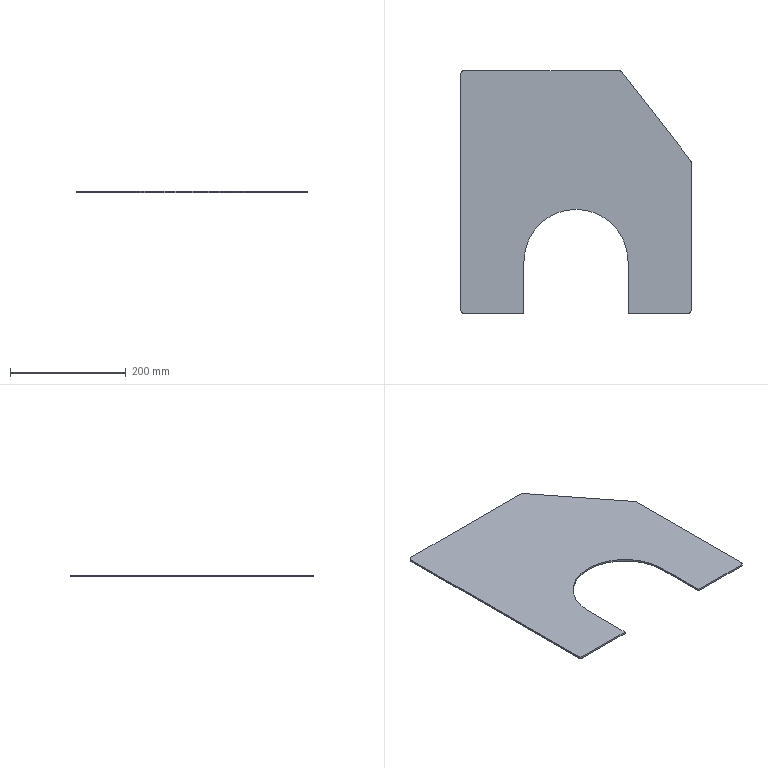Part | SolidWorks | features Extrusion 1 | 1 solid | 16 faces | box 398 x 420 x 3 mm | volume 386101 mm3 | plane 10 | cylinder 6 | commonest cylinder face diameters 10 x5 180 x1
STEP:
#1=CARTESIAN_POINT('',(0.,5.,0.));
#2=VERTEX_POINT('',#1);
#3=CARTESIAN_POINT('',(5.,0.,0.));
#4=VERTEX_POINT('',#3);
#5=CARTESIAN_POINT('',(5.,5.,0.));
#6=DIRECTION('',(0.,0.,1.));
#7=DIRECTION('',(1.,0.,0.));
#8=AXIS2_PLACEMENT_3D('',#5,#6,#7);
#9=CIRCLE('',#8,5.);
#10=EDGE_CURVE('',#2,#4,#9,.T.);
#11=ORIENTED_EDGE('',*,*,#10,.T.);
#12=CARTESIAN_POINT('',(5.,0.,3.));
#13=VERTEX_POINT('',#12);
#14=CARTESIAN_POINT('',(5.,0.,3.));
#15=DIRECTION('',(0.,0.,-1.));
#16=VECTOR('',#15,1000.);
#17=LINE('',#14,#16);
#18=EDGE_CURVE('',#13,#4,#17,.T.);
#19=ORIENTED_EDGE('',*,*,#18,.F.);
#20=CARTESIAN_POINT('',(0.,5.,3.));
#21=VERTEX_POINT('',#20);
#22=CARTESIAN_POINT('',(5.,5.,3.));
#23=DIRECTION('',(0.,0.,1.));
#24=DIRECTION('',(1.,0.,0.));
#25=AXIS2_PLACEMENT_3D('',#22,#23,#24);
#26=CIRCLE('',#25,5.);
#27=EDGE_CURVE('',#21,#13,#26,.T.);
#28=ORIENTED_EDGE('',*,*,#27,.F.);
#29=CARTESIAN_POINT('',(0.,5.,3.));
#30=DIRECTION('',(0.,0.,-1.));
#31=VECTOR('',#30,1000.);
#32=LINE('',#29,#31);
#33=EDGE_CURVE('',#21,#2,#32,.T.);
#34=ORIENTED_EDGE('',*,*,#33,.T.);
#35=EDGE_LOOP('',(#11,#19,#28,#34));
#36=FACE_OUTER_BOUND('',#35,.T.);
#37=CARTESIAN_POINT('',(5.,5.,3.));
#38=DIRECTION('',(0.,0.,-1.));
#39=DIRECTION('',(-1.,0.,0.));
#40=AXIS2_PLACEMENT_3D('',#37,#38,#39);
#41=CYLINDRICAL_SURFACE('',#40,5.);
#42=ADVANCED_FACE('',(#36),#41,.T.);
#43=CARTESIAN_POINT('',(109.,0.,0.));
#44=VERTEX_POINT('',#43);
#45=CARTESIAN_POINT('',(109.,0.,0.));
#46=DIRECTION('',(1.,0.,0.));
#47=VECTOR('',#46,1000.);
#48=LINE('',#45,#47);
#49=EDGE_CURVE('',#4,#44,#48,.T.);
#50=ORIENTED_EDGE('',*,*,#49,.T.);
#51=CARTESIAN_POINT('',(109.,0.,3.));
#52=VERTEX_POINT('',#51);
#53=CARTESIAN_POINT('',(109.,0.,3.));
#54=DIRECTION('',(0.,0.,-1.));
#55=VECTOR('',#54,1000.);
#56=LINE('',#53,#55);
#57=EDGE_CURVE('',#52,#44,#56,.T.);
#58=ORIENTED_EDGE('',*,*,#57,.F.);
#59=CARTESIAN_POINT('',(109.,0.,3.));
#60=DIRECTION('',(1.,0.,0.));
#61=VECTOR('',#60,1000.);
#62=LINE('',#59,#61);
#63=EDGE_CURVE('',#13,#52,#62,.T.);
#64=ORIENTED_EDGE('',*,*,#63,.F.);
#65=ORIENTED_EDGE('',*,*,#18,.T.);
#66=EDGE_LOOP('',(#50,#58,#64,#65));
#67=FACE_OUTER_BOUND('',#66,.T.);
#68=CARTESIAN_POINT('',(109.,0.,3.));
#69=DIRECTION('',(0.,1.,0.));
#70=DIRECTION('',(-1.,0.,0.));
#71=AXIS2_PLACEMENT_3D('',#68,#69,#70);
#72=PLANE('',#71);
#73=ADVANCED_FACE('',(#67),#72,.F.);
#74=CARTESIAN_POINT('',(109.,90.,0.));
#75=VERTEX_POINT('',#74);
#76=CARTESIAN_POINT('',(109.,90.,0.));
#77=DIRECTION('',(0.,1.,0.));
#78=VECTOR('',#77,1000.);
#79=LINE('',#76,#78);
#80=EDGE_CURVE('',#44,#75,#79,.T.);
#81=ORIENTED_EDGE('',*,*,#80,.T.);
#82=CARTESIAN_POINT('',(109.,90.,3.));
#83=VERTEX_POINT('',#82);
#84=CARTESIAN_POINT('',(109.,90.,3.));
#85=DIRECTION('',(0.,0.,-1.));
#86=VECTOR('',#85,1000.);
#87=LINE('',#84,#86);
#88=EDGE_CURVE('',#83,#75,#87,.T.);
#89=ORIENTED_EDGE('',*,*,#88,.F.);
#90=CARTESIAN_POINT('',(109.,90.,3.));
#91=DIRECTION('',(0.,1.,0.));
#92=VECTOR('',#91,1000.);
#93=LINE('',#90,#92);
#94=EDGE_CURVE('',#52,#83,#93,.T.);
#95=ORIENTED_EDGE('',*,*,#94,.F.);
#96=ORIENTED_EDGE('',*,*,#57,.T.);
#97=EDGE_LOOP('',(#81,#89,#95,#96));
#98=FACE_OUTER_BOUND('',#97,.T.);
#99=CARTESIAN_POINT('',(109.,90.,3.));
#100=DIRECTION('',(-1.,0.,0.));
#101=DIRECTION('',(0.,-1.,0.));
#102=AXIS2_PLACEMENT_3D('',#99,#100,#101);
#103=PLANE('',#102);
#104=ADVANCED_FACE('',(#98),#103,.F.);
#105=CARTESIAN_POINT('',(289.,90.,0.));
#106=VERTEX_POINT('',#105);
#107=CARTESIAN_POINT('',(199.,90.,0.));
#108=DIRECTION('',(0.,0.,-1.));
#109=DIRECTION('',(1.,0.,0.));
#110=AXIS2_PLACEMENT_3D('',#107,#108,#109);
#111=CIRCLE('',#110,90.);
#112=EDGE_CURVE('',#75,#106,#111,.T.);
#113=ORIENTED_EDGE('',*,*,#112,.T.);
#114=CARTESIAN_POINT('',(289.,90.,3.));
#115=VERTEX_POINT('',#114);
#116=CARTESIAN_POINT('',(289.,90.,3.));
#117=DIRECTION('',(0.,0.,-1.));
#118=VECTOR('',#117,1000.);
#119=LINE('',#116,#118);
#120=EDGE_CURVE('',#115,#106,#119,.T.);
#121=ORIENTED_EDGE('',*,*,#120,.F.);
#122=CARTESIAN_POINT('',(199.,90.,3.));
#123=DIRECTION('',(0.,0.,-1.));
#124=DIRECTION('',(1.,0.,0.));
#125=AXIS2_PLACEMENT_3D('',#122,#123,#124);
#126=CIRCLE('',#125,90.);
#127=EDGE_CURVE('',#83,#115,#126,.T.);
#128=ORIENTED_EDGE('',*,*,#127,.F.);
#129=ORIENTED_EDGE('',*,*,#88,.T.);
#130=EDGE_LOOP('',(#113,#121,#128,#129));
#131=FACE_OUTER_BOUND('',#130,.T.);
#132=CARTESIAN_POINT('',(199.,90.,3.));
#133=DIRECTION('',(0.,0.,-1.));
#134=DIRECTION('',(-1.,0.,0.));
#135=AXIS2_PLACEMENT_3D('',#132,#133,#134);
#136=CYLINDRICAL_SURFACE('',#135,90.);
#137=ADVANCED_FACE('',(#131),#136,.F.);
#138=CARTESIAN_POINT('',(289.,0.,0.));
#139=VERTEX_POINT('',#138);
#140=CARTESIAN_POINT('',(289.,90.,0.));
#141=DIRECTION('',(0.,-1.,0.));
#142=VECTOR('',#141,1000.);
#143=LINE('',#140,#142);
#144=EDGE_CURVE('',#106,#139,#143,.T.);
#145=ORIENTED_EDGE('',*,*,#144,.T.);
#146=CARTESIAN_POINT('',(289.,0.,3.));
#147=VERTEX_POINT('',#146);
#148=CARTESIAN_POINT('',(289.,0.,3.));
#149=DIRECTION('',(0.,0.,-1.));
#150=VECTOR('',#149,1000.);
#151=LINE('',#148,#150);
#152=EDGE_CURVE('',#147,#139,#151,.T.);
#153=ORIENTED_EDGE('',*,*,#152,.F.);
#154=CARTESIAN_POINT('',(289.,90.,3.));
#155=DIRECTION('',(0.,-1.,0.));
#156=VECTOR('',#155,1000.);
#157=LINE('',#154,#156);
#158=EDGE_CURVE('',#115,#147,#157,.T.);
#159=ORIENTED_EDGE('',*,*,#158,.F.);
#160=ORIENTED_EDGE('',*,*,#120,.T.);
#161=EDGE_LOOP('',(#145,#153,#159,#160));
#162=FACE_OUTER_BOUND('',#161,.T.);
#163=CARTESIAN_POINT('',(289.,90.,3.));
#164=DIRECTION('',(1.,0.,0.));
#165=DIRECTION('',(0.,0.,-1.));
#166=AXIS2_PLACEMENT_3D('',#163,#164,#165);
#167=PLANE('',#166);
#168=ADVANCED_FACE('',(#162),#167,.F.);
#169=CARTESIAN_POINT('',(393.,0.,0.));
#170=VERTEX_POINT('',#169);
#171=CARTESIAN_POINT('',(393.,0.,0.));
#172=DIRECTION('',(1.,0.,0.));
#173=VECTOR('',#172,1000.);
#174=LINE('',#171,#173);
#175=EDGE_CURVE('',#139,#170,#174,.T.);
#176=ORIENTED_EDGE('',*,*,#175,.T.);
#177=CARTESIAN_POINT('',(393.,0.,3.));
#178=VERTEX_POINT('',#177);
#179=CARTESIAN_POINT('',(393.,0.,3.));
#180=DIRECTION('',(0.,0.,-1.));
#181=VECTOR('',#180,1000.);
#182=LINE('',#179,#181);
#183=EDGE_CURVE('',#178,#170,#182,.T.);
#184=ORIENTED_EDGE('',*,*,#183,.F.);
#185=CARTESIAN_POINT('',(393.,0.,3.));
#186=DIRECTION('',(1.,0.,0.));
#187=VECTOR('',#186,1000.);
#188=LINE('',#185,#187);
#189=EDGE_CURVE('',#147,#178,#188,.T.);
#190=ORIENTED_EDGE('',*,*,#189,.F.);
#191=ORIENTED_EDGE('',*,*,#152,.T.);
#192=EDGE_LOOP('',(#176,#184,#190,#191));
#193=FACE_OUTER_BOUND('',#192,.T.);
#194=CARTESIAN_POINT('',(393.,0.,3.));
#195=DIRECTION('',(0.,1.,0.));
#196=DIRECTION('',(-1.,0.,0.));
#197=AXIS2_PLACEMENT_3D('',#194,#195,#196);
#198=PLANE('',#197);
#199=ADVANCED_FACE('',(#193),#198,.F.);
#200=CARTESIAN_POINT('',(398.,5.,0.));
#201=VERTEX_POINT('',#200);
#202=CARTESIAN_POINT('',(393.,5.,0.));
#203=DIRECTION('',(0.,0.,1.));
#204=DIRECTION('',(-1.,0.,0.));
#205=AXIS2_PLACEMENT_3D('',#202,#203,#204);
#206=CIRCLE('',#205,5.);
#207=EDGE_CURVE('',#170,#201,#206,.T.);
#208=ORIENTED_EDGE('',*,*,#207,.T.);
#209=CARTESIAN_POINT('',(398.,5.,3.));
#210=VERTEX_POINT('',#209);
#211=CARTESIAN_POINT('',(398.,5.,3.));
#212=DIRECTION('',(0.,0.,-1.));
#213=VECTOR('',#212,1000.);
#214=LINE('',#211,#213);
#215=EDGE_CURVE('',#210,#201,#214,.T.);
#216=ORIENTED_EDGE('',*,*,#215,.F.);
#217=CARTESIAN_POINT('',(393.,5.,3.));
#218=DIRECTION('',(0.,0.,1.));
#219=DIRECTION('',(-1.,0.,0.));
#220=AXIS2_PLACEMENT_3D('',#217,#218,#219);
#221=CIRCLE('',#220,5.);
#222=EDGE_CURVE('',#178,#210,#221,.T.);
#223=ORIENTED_EDGE('',*,*,#222,.F.);
#224=ORIENTED_EDGE('',*,*,#183,.T.);
#225=EDGE_LOOP('',(#208,#216,#223,#224));
#226=FACE_OUTER_BOUND('',#225,.T.);
#227=CARTESIAN_POINT('',(393.,5.,3.));
#228=DIRECTION('',(0.,0.,-1.));
#229=DIRECTION('',(-1.,0.,0.));
#230=AXIS2_PLACEMENT_3D('',#227,#228,#229);
#231=CYLINDRICAL_SURFACE('',#230,5.);
#232=ADVANCED_FACE('',(#226),#231,.T.);
#233=CARTESIAN_POINT('',(398.,262.178,0.));
#234=VERTEX_POINT('',#233);
#235=CARTESIAN_POINT('',(398.,262.178,0.));
#236=DIRECTION('',(0.,1.,0.));
#237=VECTOR('',#236,1000.);
#238=LINE('',#235,#237);
#239=EDGE_CURVE('',#201,#234,#238,.T.);
#240=ORIENTED_EDGE('',*,*,#239,.T.);
#241=CARTESIAN_POINT('',(398.,262.178,3.));
#242=VERTEX_POINT('',#241);
#243=CARTESIAN_POINT('',(398.,262.178,3.));
#244=DIRECTION('',(0.,0.,-1.));
#245=VECTOR('',#244,1000.);
#246=LINE('',#243,#245);
#247=EDGE_CURVE('',#242,#234,#246,.T.);
#248=ORIENTED_EDGE('',*,*,#247,.F.);
#249=CARTESIAN_POINT('',(398.,262.178,3.));
#250=DIRECTION('',(0.,1.,0.));
#251=VECTOR('',#250,1000.);
#252=LINE('',#249,#251);
#253=EDGE_CURVE('',#210,#242,#252,.T.);
#254=ORIENTED_EDGE('',*,*,#253,.F.);
#255=ORIENTED_EDGE('',*,*,#215,.T.);
#256=EDGE_LOOP('',(#240,#248,#254,#255));
#257=FACE_OUTER_BOUND('',#256,.T.);
#258=CARTESIAN_POINT('',(398.,262.178,3.));
#259=DIRECTION('',(-1.,0.,0.));
#260=DIRECTION('',(0.,-1.,0.));
#261=AXIS2_PLACEMENT_3D('',#258,#259,#260);
#262=PLANE('',#261);
#263=ADVANCED_FACE('',(#257),#262,.F.);
#264=CARTESIAN_POINT('',(396.94,265.257,0.));
#265=VERTEX_POINT('',#264);
#266=CARTESIAN_POINT('',(393.,262.178,0.));
#267=DIRECTION('',(0.,0.,1.));
#268=DIRECTION('',(-1.,0.,0.));
#269=AXIS2_PLACEMENT_3D('',#266,#267,#268);
#270=CIRCLE('',#269,5.);
#271=EDGE_CURVE('',#234,#265,#270,.T.);
#272=ORIENTED_EDGE('',*,*,#271,.T.);
#273=CARTESIAN_POINT('',(396.94,265.257,3.));
#274=VERTEX_POINT('',#273);
#275=CARTESIAN_POINT('',(396.94,265.257,3.));
#276=DIRECTION('',(0.,0.,-1.));
#277=VECTOR('',#276,1000.);
#278=LINE('',#275,#277);
#279=EDGE_CURVE('',#274,#265,#278,.T.);
#280=ORIENTED_EDGE('',*,*,#279,.F.);
#281=CARTESIAN_POINT('',(393.,262.178,3.));
#282=DIRECTION('',(0.,0.,1.));
#283=DIRECTION('',(-1.,0.,0.));
#284=AXIS2_PLACEMENT_3D('',#281,#282,#283);
#285=CIRCLE('',#284,5.);
#286=EDGE_CURVE('',#242,#274,#285,.T.);
#287=ORIENTED_EDGE('',*,*,#286,.F.);
#288=ORIENTED_EDGE('',*,*,#247,.T.);
#289=EDGE_LOOP('',(#272,#280,#287,#288));
#290=FACE_OUTER_BOUND('',#289,.T.);
#291=CARTESIAN_POINT('',(393.,262.178,3.));
#292=DIRECTION('',(0.,0.,-1.));
#293=DIRECTION('',(-1.,0.,0.));
#294=AXIS2_PLACEMENT_3D('',#291,#292,#293);
#295=CYLINDRICAL_SURFACE('',#294,5.);
#296=ADVANCED_FACE('',(#290),#295,.T.);
#297=CARTESIAN_POINT('',(277.543,418.078,0.));
#298=VERTEX_POINT('',#297);
#299=CARTESIAN_POINT('',(277.543,418.078,0.));
#300=DIRECTION('',(-0.6157,0.788,0.));
#301=VECTOR('',#300,1000.);
#302=LINE('',#299,#301);
#303=EDGE_CURVE('',#265,#298,#302,.T.);
#304=ORIENTED_EDGE('',*,*,#303,.T.);
#305=CARTESIAN_POINT('',(277.543,418.078,3.));
#306=VERTEX_POINT('',#305);
#307=CARTESIAN_POINT('',(277.543,418.078,3.));
#308=DIRECTION('',(0.,0.,-1.));
#309=VECTOR('',#308,1000.);
#310=LINE('',#307,#309);
#311=EDGE_CURVE('',#306,#298,#310,.T.);
#312=ORIENTED_EDGE('',*,*,#311,.F.);
#313=CARTESIAN_POINT('',(277.543,418.078,3.));
#314=DIRECTION('',(-0.6157,0.788,0.));
#315=VECTOR('',#314,1000.);
#316=LINE('',#313,#315);
#317=EDGE_CURVE('',#274,#306,#316,.T.);
#318=ORIENTED_EDGE('',*,*,#317,.F.);
#319=ORIENTED_EDGE('',*,*,#279,.T.);
#320=EDGE_LOOP('',(#304,#312,#318,#319));
#321=FACE_OUTER_BOUND('',#320,.T.);
#322=CARTESIAN_POINT('',(277.543,418.078,3.));
#323=DIRECTION('',(-0.788,-0.6157,0.));
#324=DIRECTION('',(0.6157,-0.788,0.));
#325=AXIS2_PLACEMENT_3D('',#322,#323,#324);
#326=PLANE('',#325);
#327=ADVANCED_FACE('',(#321),#326,.F.);
#328=CARTESIAN_POINT('',(273.603,420.,0.));
#329=VERTEX_POINT('',#328);
#330=CARTESIAN_POINT('',(273.603,415.,0.));
#331=DIRECTION('',(0.,0.,1.));
#332=DIRECTION('',(-1.,0.,0.));
#333=AXIS2_PLACEMENT_3D('',#330,#331,#332);
#334=CIRCLE('',#333,5.);
#335=EDGE_CURVE('',#298,#329,#334,.T.);
#336=ORIENTED_EDGE('',*,*,#335,.T.);
#337=CARTESIAN_POINT('',(273.603,420.,3.));
#338=VERTEX_POINT('',#337);
#339=CARTESIAN_POINT('',(273.603,420.,3.));
#340=DIRECTION('',(0.,0.,-1.));
#341=VECTOR('',#340,1000.);
#342=LINE('',#339,#341);
#343=EDGE_CURVE('',#338,#329,#342,.T.);
#344=ORIENTED_EDGE('',*,*,#343,.F.);
#345=CARTESIAN_POINT('',(273.603,415.,3.));
#346=DIRECTION('',(0.,0.,1.));
#347=DIRECTION('',(-1.,0.,0.));
#348=AXIS2_PLACEMENT_3D('',#345,#346,#347);
#349=CIRCLE('',#348,5.);
#350=EDGE_CURVE('',#306,#338,#349,.T.);
#351=ORIENTED_EDGE('',*,*,#350,.F.);
#352=ORIENTED_EDGE('',*,*,#311,.T.);
#353=EDGE_LOOP('',(#336,#344,#351,#352));
#354=FACE_OUTER_BOUND('',#353,.T.);
#355=CARTESIAN_POINT('',(273.603,415.,3.));
#356=DIRECTION('',(0.,0.,-1.));
#357=DIRECTION('',(-1.,0.,0.));
#358=AXIS2_PLACEMENT_3D('',#355,#356,#357);
#359=CYLINDRICAL_SURFACE('',#358,5.);
#360=ADVANCED_FACE('',(#354),#359,.T.);
#361=CARTESIAN_POINT('',(5.,420.,0.));
#362=VERTEX_POINT('',#361);
#363=CARTESIAN_POINT('',(5.,420.,0.));
#364=DIRECTION('',(-1.,0.,0.));
#365=VECTOR('',#364,1000.);
#366=LINE('',#363,#365);
#367=EDGE_CURVE('',#329,#362,#366,.T.);
#368=ORIENTED_EDGE('',*,*,#367,.T.);
#369=CARTESIAN_POINT('',(5.,420.,3.));
#370=VERTEX_POINT('',#369);
#371=CARTESIAN_POINT('',(5.,420.,3.));
#372=DIRECTION('',(0.,0.,-1.));
#373=VECTOR('',#372,1000.);
#374=LINE('',#371,#373);
#375=EDGE_CURVE('',#370,#362,#374,.T.);
#376=ORIENTED_EDGE('',*,*,#375,.F.);
#377=CARTESIAN_POINT('',(5.,420.,3.));
#378=DIRECTION('',(-1.,0.,0.));
#379=VECTOR('',#378,1000.);
#380=LINE('',#377,#379);
#381=EDGE_CURVE('',#338,#370,#380,.T.);
#382=ORIENTED_EDGE('',*,*,#381,.F.);
#383=ORIENTED_EDGE('',*,*,#343,.T.);
#384=EDGE_LOOP('',(#368,#376,#382,#383));
#385=FACE_OUTER_BOUND('',#384,.T.);
#386=CARTESIAN_POINT('',(5.,420.,3.));
#387=DIRECTION('',(0.,-1.,0.));
#388=DIRECTION('',(0.,0.,-1.));
#389=AXIS2_PLACEMENT_3D('',#386,#387,#388);
#390=PLANE('',#389);
#391=ADVANCED_FACE('',(#385),#390,.F.);
#392=CARTESIAN_POINT('',(0.,415.,0.));
#393=VERTEX_POINT('',#392);
#394=CARTESIAN_POINT('',(5.,415.,0.));
#395=DIRECTION('',(0.,0.,1.));
#396=DIRECTION('',(-1.,0.,0.));
#397=AXIS2_PLACEMENT_3D('',#394,#395,#396);
#398=CIRCLE('',#397,5.);
#399=EDGE_CURVE('',#362,#393,#398,.T.);
#400=ORIENTED_EDGE('',*,*,#399,.T.);
#401=CARTESIAN_POINT('',(0.,415.,3.));
#402=VERTEX_POINT('',#401);
#403=CARTESIAN_POINT('',(0.,415.,3.));
#404=DIRECTION('',(0.,0.,-1.));
#405=VECTOR('',#404,1000.);
#406=LINE('',#403,#405);
#407=EDGE_CURVE('',#402,#393,#406,.T.);
#408=ORIENTED_EDGE('',*,*,#407,.F.);
#409=CARTESIAN_POINT('',(5.,415.,3.));
#410=DIRECTION('',(0.,0.,1.));
#411=DIRECTION('',(-1.,0.,0.));
#412=AXIS2_PLACEMENT_3D('',#409,#410,#411);
#413=CIRCLE('',#412,5.);
#414=EDGE_CURVE('',#370,#402,#413,.T.);
#415=ORIENTED_EDGE('',*,*,#414,.F.);
#416=ORIENTED_EDGE('',*,*,#375,.T.);
#417=EDGE_LOOP('',(#400,#408,#415,#416));
#418=FACE_OUTER_BOUND('',#417,.T.);
#419=CARTESIAN_POINT('',(5.,415.,3.));
#420=DIRECTION('',(0.,0.,-1.));
#421=DIRECTION('',(-1.,0.,0.));
#422=AXIS2_PLACEMENT_3D('',#419,#420,#421);
#423=CYLINDRICAL_SURFACE('',#422,5.);
#424=ADVANCED_FACE('',(#418),#423,.T.);
#425=CARTESIAN_POINT('',(0.,5.,0.));
#426=DIRECTION('',(0.,-1.,0.));
#427=VECTOR('',#426,1000.);
#428=LINE('',#425,#427);
#429=EDGE_CURVE('',#393,#2,#428,.T.);
#430=ORIENTED_EDGE('',*,*,#429,.T.);
#431=ORIENTED_EDGE('',*,*,#33,.F.);
#432=CARTESIAN_POINT('',(0.,5.,3.));
#433=DIRECTION('',(0.,-1.,0.));
#434=VECTOR('',#433,1000.);
#435=LINE('',#432,#434);
#436=EDGE_CURVE('',#402,#21,#435,.T.);
#437=ORIENTED_EDGE('',*,*,#436,.F.);
#438=ORIENTED_EDGE('',*,*,#407,.T.);
#439=EDGE_LOOP('',(#430,#431,#437,#438));
#440=FACE_OUTER_BOUND('',#439,.T.);
#441=CARTESIAN_POINT('',(0.,5.,3.));
#442=DIRECTION('',(1.,0.,0.));
#443=DIRECTION('',(0.,0.,-1.));
#444=AXIS2_PLACEMENT_3D('',#441,#442,#443);
#445=PLANE('',#444);
#446=ADVANCED_FACE('',(#440),#445,.F.);
#447=ORIENTED_EDGE('',*,*,#27,.T.);
#448=ORIENTED_EDGE('',*,*,#63,.T.);
#449=ORIENTED_EDGE('',*,*,#94,.T.);
#450=ORIENTED_EDGE('',*,*,#127,.T.);
#451=ORIENTED_EDGE('',*,*,#158,.T.);
#452=ORIENTED_EDGE('',*,*,#189,.T.);
#453=ORIENTED_EDGE('',*,*,#222,.T.);
#454=ORIENTED_EDGE('',*,*,#253,.T.);
#455=ORIENTED_EDGE('',*,*,#286,.T.);
#456=ORIENTED_EDGE('',*,*,#317,.T.);
#457=ORIENTED_EDGE('',*,*,#350,.T.);
#458=ORIENTED_EDGE('',*,*,#381,.T.);
#459=ORIENTED_EDGE('',*,*,#414,.T.);
#460=ORIENTED_EDGE('',*,*,#436,.T.);
#461=EDGE_LOOP('',(#447,#448,#449,#450,#451,#452,#453,#454,#455,#456,#457,#458,#459,#460));
#462=FACE_OUTER_BOUND('',#461,.T.);
#463=CARTESIAN_POINT('',(5.,5.,3.));
#464=DIRECTION('',(0.,0.,1.));
#465=DIRECTION('',(1.,0.,0.));
#466=AXIS2_PLACEMENT_3D('',#463,#464,#465);
#467=PLANE('',#466);
#468=ADVANCED_FACE('',(#462),#467,.T.);
#469=ORIENTED_EDGE('',*,*,#10,.F.);
#470=ORIENTED_EDGE('',*,*,#429,.F.);
#471=ORIENTED_EDGE('',*,*,#399,.F.);
#472=ORIENTED_EDGE('',*,*,#367,.F.);
#473=ORIENTED_EDGE('',*,*,#335,.F.);
#474=ORIENTED_EDGE('',*,*,#303,.F.);
#475=ORIENTED_EDGE('',*,*,#271,.F.);
#476=ORIENTED_EDGE('',*,*,#239,.F.);
#477=ORIENTED_EDGE('',*,*,#207,.F.);
#478=ORIENTED_EDGE('',*,*,#175,.F.);
#479=ORIENTED_EDGE('',*,*,#144,.F.);
#480=ORIENTED_EDGE('',*,*,#112,.F.);
#481=ORIENTED_EDGE('',*,*,#80,.F.);
#482=ORIENTED_EDGE('',*,*,#49,.F.);
#483=EDGE_LOOP('',(#469,#470,#471,#472,#473,#474,#475,#476,#477,#478,#479,#480,#481,#482));
#484=FACE_OUTER_BOUND('',#483,.T.);
#485=CARTESIAN_POINT('',(5.,5.,0.));
#486=DIRECTION('',(0.,0.,1.));
#487=DIRECTION('',(1.,0.,0.));
#488=AXIS2_PLACEMENT_3D('',#485,#486,#487);
#489=PLANE('',#488);
#490=ADVANCED_FACE('',(#484),#489,.F.);
#491=CLOSED_SHELL('',(#42,#73,#104,#137,#168,#199,#232,#263,#296,#327,#360,#391,#424,#446,#468,#490));
#492=MANIFOLD_SOLID_BREP('',#491);
#493=CARTESIAN_POINT('',(0.,0.,0.));
#494=DIRECTION('',(0.,0.,1.));
#495=DIRECTION('',(1.,0.,0.));
#496=AXIS2_PLACEMENT_3D('',#493,#494,#495);
#497=(LENGTH_UNIT()NAMED_UNIT(*)SI_UNIT(.MILLI.,.METRE.));
#498=UNCERTAINTY_MEASURE_WITH_UNIT(LENGTH_MEASURE(0.00001),#497,'','');
#499=(NAMED_UNIT(*)PLANE_ANGLE_UNIT()SI_UNIT($,.RADIAN.));
#500=(NAMED_UNIT(*)SI_UNIT($,.STERADIAN.)SOLID_ANGLE_UNIT());
#501=(GEOMETRIC_REPRESENTATION_CONTEXT(3)GLOBAL_UNCERTAINTY_ASSIGNED_CONTEXT((#498))GLOBAL_UNIT_ASSIGNED_CONTEXT((#497,#499,#500))REPRESENTATION_CONTEXT('',''));
#502=ADVANCED_BREP_SHAPE_REPRESENTATION('',(#492,#496),#501);